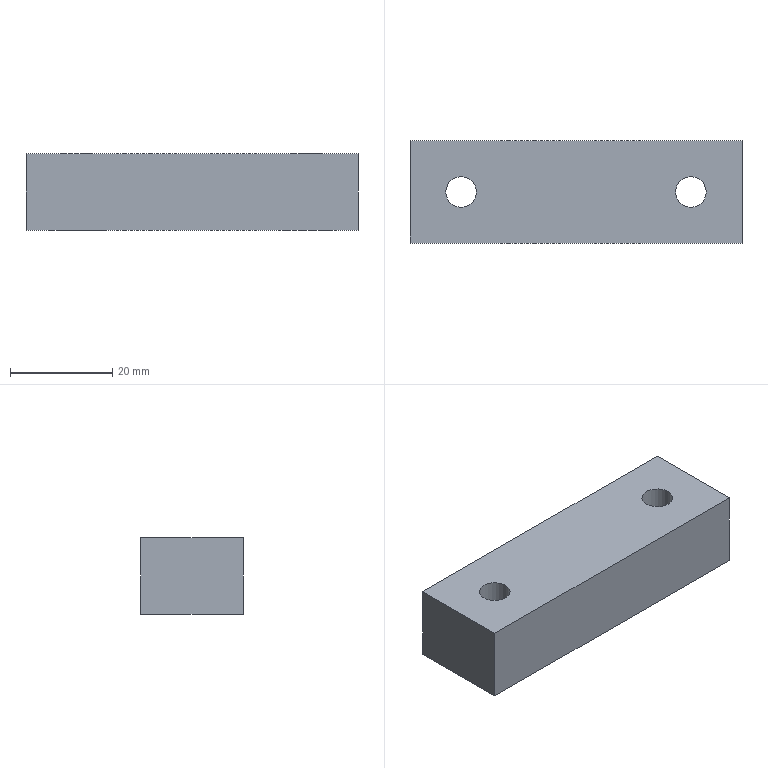Part | STEP file | gslz 2016.10.28-10_id2114_x_t | 1 solid | 12 faces | box 65 x 20 x 15 mm | volume 17584 mm3 | plane 8 | cylinder 4 | commonest cylinder face diameters 6 x2 11 x2
STEP:
#1=CARTESIAN_POINT('',(0.,0.,0.));
#2=DIRECTION('',(0.,0.,1.));
#3=DIRECTION('',(1.,0.,0.));
#4=AXIS2_PLACEMENT_3D('',#1,#2,#3);
#5=CARTESIAN_POINT('',(-46.5,-250.,28.));
#6=VERTEX_POINT('',#5);
#7=CARTESIAN_POINT('',(-41.,-250.,28.));
#8=DIRECTION('',(0.,0.,-1.));
#9=DIRECTION('',(-1.,0.,0.));
#10=AXIS2_PLACEMENT_3D('',#7,#8,#9);
#11=CIRCLE('',#10,5.5);
#12=CARTESIAN_POINT('',(-41.,-250.,30.));
#13=DIRECTION('',(0.,0.,-1.));
#14=DIRECTION('',(-1.,0.,0.));
#15=AXIS2_PLACEMENT_3D('',#12,#13,#14);
#16=CYLINDRICAL_SURFACE('',#15,5.5);
#17=CARTESIAN_POINT('',(0.,2.));
#18=DIRECTION('',(1.,0.));
#19=VECTOR('',#18,1.);
#20=LINE('',#17,#19);
#21=(GEOMETRIC_REPRESENTATION_CONTEXT(2)PARAMETRIC_REPRESENTATION_CONTEXT()REPRESENTATION_CONTEXT('',''));
#22=DEFINITIONAL_REPRESENTATION('',(#20),#21);
#23=PCURVE('',#16,#22);
#24=CARTESIAN_POINT('',(-3.5,-250.,28.));
#25=DIRECTION('',(0.,0.,-1.));
#26=DIRECTION('',(1.,0.,0.));
#27=AXIS2_PLACEMENT_3D('',#24,#25,#26);
#28=PLANE('',#27);
#29=CARTESIAN_POINT('',(-37.5,0.));
#30=DIRECTION('',(-1.,0.));
#31=AXIS2_PLACEMENT_2D('',#29,#30);
#32=CIRCLE('',#31,5.5);
#33=(GEOMETRIC_REPRESENTATION_CONTEXT(2)PARAMETRIC_REPRESENTATION_CONTEXT()REPRESENTATION_CONTEXT('',''));
#34=DEFINITIONAL_REPRESENTATION('',(#32),#33);
#35=PCURVE('',#28,#34);
#36=SURFACE_CURVE('',#11,(#23,#35),.PCURVE_S1.);
#37=EDGE_CURVE('',#6,#6,#36,.T.);
#38=ORIENTED_EDGE('',*,*,#37,.T.);
#39=CARTESIAN_POINT('',(-46.5,-250.,20.));
#40=VERTEX_POINT('',#39);
#41=CARTESIAN_POINT('',(-46.5,-250.,28.));
#42=CARTESIAN_POINT('',(-46.5,-250.,20.));
#43=B_SPLINE_CURVE_WITH_KNOTS('',1,(#41,#42),.UNSPECIFIED.,.F.,.F.,(2,2),(2.,10.),.PIECEWISE_BEZIER_KNOTS.);
#44=CARTESIAN_POINT('',(6.283,0.));
#45=DIRECTION('',(0.,1.));
#46=VECTOR('',#45,1.);
#47=LINE('',#44,#46);
#48=(GEOMETRIC_REPRESENTATION_CONTEXT(2)PARAMETRIC_REPRESENTATION_CONTEXT()REPRESENTATION_CONTEXT('',''));
#49=DEFINITIONAL_REPRESENTATION('',(#47),#48);
#50=PCURVE('',#16,#49);
#51=CARTESIAN_POINT('',(0.,0.));
#52=DIRECTION('',(0.,1.));
#53=VECTOR('',#52,1.);
#54=LINE('',#51,#53);
#55=(GEOMETRIC_REPRESENTATION_CONTEXT(2)PARAMETRIC_REPRESENTATION_CONTEXT()REPRESENTATION_CONTEXT('',''));
#56=DEFINITIONAL_REPRESENTATION('',(#54),#55);
#57=PCURVE('',#16,#56);
#58=SEAM_CURVE('',#43,(#50,#57),.PCURVE_S1.);
#59=EDGE_CURVE('',#6,#40,#58,.T.);
#60=ORIENTED_EDGE('',*,*,#59,.T.);
#61=CARTESIAN_POINT('',(-35.5,-250.,20.));
#62=VERTEX_POINT('',#61);
#63=CARTESIAN_POINT('',(-41.,-250.,20.));
#64=DIRECTION('',(0.,0.,-1.));
#65=DIRECTION('',(1.,0.,0.));
#66=AXIS2_PLACEMENT_3D('',#63,#64,#65);
#67=CIRCLE('',#66,5.5);
#68=CARTESIAN_POINT('',(3.142,10.));
#69=DIRECTION('',(1.,0.));
#70=VECTOR('',#69,1.);
#71=LINE('',#68,#70);
#72=(GEOMETRIC_REPRESENTATION_CONTEXT(2)PARAMETRIC_REPRESENTATION_CONTEXT()REPRESENTATION_CONTEXT('',''));
#73=DEFINITIONAL_REPRESENTATION('',(#71),#72);
#74=PCURVE('',#16,#73);
#75=CARTESIAN_POINT('',(-193.5,-250.,20.));
#76=DIRECTION('',(0.,0.,1.));
#77=DIRECTION('',(1.,0.,0.));
#78=AXIS2_PLACEMENT_3D('',#75,#76,#77);
#79=PLANE('',#78);
#80=CARTESIAN_POINT('',(158.,0.));
#81=CARTESIAN_POINT('',(158.,-9.526));
#82=CARTESIAN_POINT('',(149.75,-4.763));
#83=CARTESIAN_POINT('',(141.5,0.));
#84=CARTESIAN_POINT('',(149.75,4.763));
#85=CARTESIAN_POINT('',(158.,9.526));
#86=CARTESIAN_POINT('',(158.,0.));
#87=(BOUNDED_CURVE()B_SPLINE_CURVE(2,(#80,#81,#82,#83,#84,#85,#86),.UNSPECIFIED.,.T.,.F.)B_SPLINE_CURVE_WITH_KNOTS((1,2,2,2,2,1),(-2.094,0.,2.094,4.189,6.283,8.378),.UNSPECIFIED.)CURVE()GEOMETRIC_REPRESENTATION_ITEM()RATIONAL_B_SPLINE_CURVE((1.,0.5,1.,0.5,1.,0.5,1.))REPRESENTATION_ITEM(''));
#88=(GEOMETRIC_REPRESENTATION_CONTEXT(2)PARAMETRIC_REPRESENTATION_CONTEXT()REPRESENTATION_CONTEXT('',''));
#89=DEFINITIONAL_REPRESENTATION('',(#87),#88);
#90=PCURVE('',#79,#89);
#91=SURFACE_CURVE('',#67,(#74,#90),.PCURVE_S1.);
#92=EDGE_CURVE('',#62,#40,#91,.T.);
#93=ORIENTED_EDGE('',*,*,#92,.F.);
#94=CARTESIAN_POINT('',(-41.,-250.,20.));
#95=DIRECTION('',(0.,0.,-1.));
#96=DIRECTION('',(1.,0.,0.));
#97=AXIS2_PLACEMENT_3D('',#94,#95,#96);
#98=CIRCLE('',#97,5.5);
#99=CARTESIAN_POINT('',(-3.142,10.));
#100=DIRECTION('',(1.,0.));
#101=VECTOR('',#100,1.);
#102=LINE('',#99,#101);
#103=(GEOMETRIC_REPRESENTATION_CONTEXT(2)PARAMETRIC_REPRESENTATION_CONTEXT()REPRESENTATION_CONTEXT('',''));
#104=DEFINITIONAL_REPRESENTATION('',(#102),#103);
#105=PCURVE('',#16,#104);
#106=CARTESIAN_POINT('',(158.,0.));
#107=CARTESIAN_POINT('',(158.,-9.526));
#108=CARTESIAN_POINT('',(149.75,-4.763));
#109=CARTESIAN_POINT('',(141.5,0.));
#110=CARTESIAN_POINT('',(149.75,4.763));
#111=CARTESIAN_POINT('',(158.,9.526));
#112=CARTESIAN_POINT('',(158.,0.));
#113=(BOUNDED_CURVE()B_SPLINE_CURVE(2,(#106,#107,#108,#109,#110,#111,#112),.UNSPECIFIED.,.T.,.F.)B_SPLINE_CURVE_WITH_KNOTS((1,2,2,2,2,1),(-2.094,0.,2.094,4.189,6.283,8.378),.UNSPECIFIED.)CURVE()GEOMETRIC_REPRESENTATION_ITEM()RATIONAL_B_SPLINE_CURVE((1.,0.5,1.,0.5,1.,0.5,1.))REPRESENTATION_ITEM(''));
#114=(GEOMETRIC_REPRESENTATION_CONTEXT(2)PARAMETRIC_REPRESENTATION_CONTEXT()REPRESENTATION_CONTEXT('',''));
#115=DEFINITIONAL_REPRESENTATION('',(#113),#114);
#116=PCURVE('',#79,#115);
#117=SURFACE_CURVE('',#98,(#105,#116),.PCURVE_S1.);
#118=EDGE_CURVE('',#40,#62,#117,.T.);
#119=ORIENTED_EDGE('',*,*,#118,.F.);
#120=ORIENTED_EDGE('',*,*,#59,.F.);
#121=EDGE_LOOP('',(#38,#60,#93,#119,#120));
#122=FACE_BOUND('',#121,.F.);
#123=ADVANCED_FACE('',(#122),#16,.F.);
#124=CARTESIAN_POINT('',(-51.,-260.,35.));
#125=VERTEX_POINT('',#124);
#126=CARTESIAN_POINT('',(-51.,-260.,20.));
#127=VERTEX_POINT('',#126);
#128=CARTESIAN_POINT('',(-51.,-260.,30.));
#129=DIRECTION('',(0.,0.,-1.));
#130=VECTOR('',#129,1.);
#131=LINE('',#128,#130);
#132=CARTESIAN_POINT('',(-73.5,-260.,30.));
#133=DIRECTION('',(0.,1.,0.));
#134=DIRECTION('',(0.,0.,-1.));
#135=AXIS2_PLACEMENT_3D('',#132,#133,#134);
#136=PLANE('',#135);
#137=CARTESIAN_POINT('',(0.,-22.5));
#138=DIRECTION('',(1.,0.));
#139=VECTOR('',#138,1.);
#140=LINE('',#137,#139);
#141=(GEOMETRIC_REPRESENTATION_CONTEXT(2)PARAMETRIC_REPRESENTATION_CONTEXT()REPRESENTATION_CONTEXT('',''));
#142=DEFINITIONAL_REPRESENTATION('',(#140),#141);
#143=PCURVE('',#136,#142);
#144=CARTESIAN_POINT('',(-51.,-262.5,30.));
#145=DIRECTION('',(1.,0.,0.));
#146=DIRECTION('',(0.,0.,-1.));
#147=AXIS2_PLACEMENT_3D('',#144,#145,#146);
#148=PLANE('',#147);
#149=CARTESIAN_POINT('',(0.,2.5));
#150=DIRECTION('',(1.,0.));
#151=VECTOR('',#150,1.);
#152=LINE('',#149,#151);
#153=(GEOMETRIC_REPRESENTATION_CONTEXT(2)PARAMETRIC_REPRESENTATION_CONTEXT()REPRESENTATION_CONTEXT('',''));
#154=DEFINITIONAL_REPRESENTATION('',(#152),#153);
#155=PCURVE('',#148,#154);
#156=SURFACE_CURVE('',#131,(#143,#155),.PCURVE_S1.);
#157=EDGE_CURVE('',#125,#127,#156,.T.);
#158=ORIENTED_EDGE('',*,*,#157,.T.);
#159=CARTESIAN_POINT('',(14.,-260.,20.));
#160=VERTEX_POINT('',#159);
#161=CARTESIAN_POINT('',(-193.5,-260.,20.));
#162=DIRECTION('',(-1.,0.,0.));
#163=VECTOR('',#162,1.);
#164=LINE('',#161,#163);
#165=CARTESIAN_POINT('',(10.,120.));
#166=DIRECTION('',(0.,1.));
#167=VECTOR('',#166,1.);
#168=LINE('',#165,#167);
#169=(GEOMETRIC_REPRESENTATION_CONTEXT(2)PARAMETRIC_REPRESENTATION_CONTEXT()REPRESENTATION_CONTEXT('',''));
#170=DEFINITIONAL_REPRESENTATION('',(#168),#169);
#171=PCURVE('',#136,#170);
#172=CARTESIAN_POINT('',(0.,-10.));
#173=DIRECTION('',(-1.,0.));
#174=VECTOR('',#173,1.);
#175=LINE('',#172,#174);
#176=(GEOMETRIC_REPRESENTATION_CONTEXT(2)PARAMETRIC_REPRESENTATION_CONTEXT()REPRESENTATION_CONTEXT('',''));
#177=DEFINITIONAL_REPRESENTATION('',(#175),#176);
#178=PCURVE('',#79,#177);
#179=SURFACE_CURVE('',#164,(#171,#178),.PCURVE_S1.);
#180=EDGE_CURVE('',#160,#127,#179,.T.);
#181=ORIENTED_EDGE('',*,*,#180,.F.);
#182=CARTESIAN_POINT('',(14.,-260.,35.));
#183=VERTEX_POINT('',#182);
#184=CARTESIAN_POINT('',(14.,-260.,30.));
#185=DIRECTION('',(0.,0.,-1.));
#186=VECTOR('',#185,1.);
#187=LINE('',#184,#186);
#188=CARTESIAN_POINT('',(0.,-87.5));
#189=DIRECTION('',(1.,0.));
#190=VECTOR('',#189,1.);
#191=LINE('',#188,#190);
#192=(GEOMETRIC_REPRESENTATION_CONTEXT(2)PARAMETRIC_REPRESENTATION_CONTEXT()REPRESENTATION_CONTEXT('',''));
#193=DEFINITIONAL_REPRESENTATION('',(#191),#192);
#194=PCURVE('',#136,#193);
#195=CARTESIAN_POINT('',(14.,-237.5,30.));
#196=DIRECTION('',(-1.,0.,0.));
#197=DIRECTION('',(0.,0.,1.));
#198=AXIS2_PLACEMENT_3D('',#195,#196,#197);
#199=PLANE('',#198);
#200=CARTESIAN_POINT('',(0.,-22.5));
#201=DIRECTION('',(-1.,0.));
#202=VECTOR('',#201,1.);
#203=LINE('',#200,#202);
#204=(GEOMETRIC_REPRESENTATION_CONTEXT(2)PARAMETRIC_REPRESENTATION_CONTEXT()REPRESENTATION_CONTEXT('',''));
#205=DEFINITIONAL_REPRESENTATION('',(#203),#204);
#206=PCURVE('',#199,#205);
#207=SURFACE_CURVE('',#187,(#194,#206),.PCURVE_S1.);
#208=EDGE_CURVE('',#183,#160,#207,.T.);
#209=ORIENTED_EDGE('',*,*,#208,.F.);
#210=CARTESIAN_POINT('',(-193.5,-260.,35.));
#211=DIRECTION('',(-1.,0.,0.));
#212=VECTOR('',#211,1.);
#213=LINE('',#210,#212);
#214=CARTESIAN_POINT('',(-5.,120.));
#215=DIRECTION('',(0.,1.));
#216=VECTOR('',#215,1.);
#217=LINE('',#214,#216);
#218=(GEOMETRIC_REPRESENTATION_CONTEXT(2)PARAMETRIC_REPRESENTATION_CONTEXT()REPRESENTATION_CONTEXT('',''));
#219=DEFINITIONAL_REPRESENTATION('',(#217),#218);
#220=PCURVE('',#136,#219);
#221=CARTESIAN_POINT('',(-193.5,-250.,35.));
#222=DIRECTION('',(0.,0.,1.));
#223=DIRECTION('',(1.,0.,0.));
#224=AXIS2_PLACEMENT_3D('',#221,#222,#223);
#225=PLANE('',#224);
#226=CARTESIAN_POINT('',(0.,-10.));
#227=DIRECTION('',(-1.,0.));
#228=VECTOR('',#227,1.);
#229=LINE('',#226,#228);
#230=(GEOMETRIC_REPRESENTATION_CONTEXT(2)PARAMETRIC_REPRESENTATION_CONTEXT()REPRESENTATION_CONTEXT('',''));
#231=DEFINITIONAL_REPRESENTATION('',(#229),#230);
#232=PCURVE('',#225,#231);
#233=SURFACE_CURVE('',#213,(#220,#232),.PCURVE_S1.);
#234=EDGE_CURVE('',#183,#125,#233,.T.);
#235=ORIENTED_EDGE('',*,*,#234,.T.);
#236=EDGE_LOOP('',(#158,#181,#209,#235));
#237=FACE_BOUND('',#236,.T.);
#238=ADVANCED_FACE('',(#237),#136,.F.);
#239=ORIENTED_EDGE('',*,*,#208,.T.);
#240=CARTESIAN_POINT('',(14.,-240.,20.));
#241=VERTEX_POINT('',#240);
#242=CARTESIAN_POINT('',(14.,-237.5,20.));
#243=DIRECTION('',(0.,-1.,0.));
#244=VECTOR('',#243,1.);
#245=LINE('',#242,#244);
#246=CARTESIAN_POINT('',(-10.,0.));
#247=DIRECTION('',(0.,-1.));
#248=VECTOR('',#247,1.);
#249=LINE('',#246,#248);
#250=(GEOMETRIC_REPRESENTATION_CONTEXT(2)PARAMETRIC_REPRESENTATION_CONTEXT()REPRESENTATION_CONTEXT('',''));
#251=DEFINITIONAL_REPRESENTATION('',(#249),#250);
#252=PCURVE('',#199,#251);
#253=CARTESIAN_POINT('',(207.5,12.5));
#254=DIRECTION('',(0.,-1.));
#255=VECTOR('',#254,1.);
#256=LINE('',#253,#255);
#257=(GEOMETRIC_REPRESENTATION_CONTEXT(2)PARAMETRIC_REPRESENTATION_CONTEXT()REPRESENTATION_CONTEXT('',''));
#258=DEFINITIONAL_REPRESENTATION('',(#256),#257);
#259=PCURVE('',#79,#258);
#260=SURFACE_CURVE('',#245,(#252,#259),.PCURVE_S1.);
#261=EDGE_CURVE('',#241,#160,#260,.T.);
#262=ORIENTED_EDGE('',*,*,#261,.F.);
#263=CARTESIAN_POINT('',(14.,-240.,35.));
#264=VERTEX_POINT('',#263);
#265=CARTESIAN_POINT('',(14.,-240.,30.));
#266=DIRECTION('',(0.,0.,-1.));
#267=VECTOR('',#266,1.);
#268=LINE('',#265,#267);
#269=CARTESIAN_POINT('',(0.,-2.5));
#270=DIRECTION('',(-1.,0.));
#271=VECTOR('',#270,1.);
#272=LINE('',#269,#271);
#273=(GEOMETRIC_REPRESENTATION_CONTEXT(2)PARAMETRIC_REPRESENTATION_CONTEXT()REPRESENTATION_CONTEXT('',''));
#274=DEFINITIONAL_REPRESENTATION('',(#272),#273);
#275=PCURVE('',#199,#274);
#276=CARTESIAN_POINT('',(-203.5,-240.,30.));
#277=DIRECTION('',(0.,-1.,0.));
#278=DIRECTION('',(0.,0.,1.));
#279=AXIS2_PLACEMENT_3D('',#276,#277,#278);
#280=PLANE('',#279);
#281=CARTESIAN_POINT('',(0.,-217.5));
#282=DIRECTION('',(-1.,0.));
#283=VECTOR('',#282,1.);
#284=LINE('',#281,#283);
#285=(GEOMETRIC_REPRESENTATION_CONTEXT(2)PARAMETRIC_REPRESENTATION_CONTEXT()REPRESENTATION_CONTEXT('',''));
#286=DEFINITIONAL_REPRESENTATION('',(#284),#285);
#287=PCURVE('',#280,#286);
#288=SURFACE_CURVE('',#268,(#275,#287),.PCURVE_S1.);
#289=EDGE_CURVE('',#264,#241,#288,.T.);
#290=ORIENTED_EDGE('',*,*,#289,.F.);
#291=CARTESIAN_POINT('',(14.,-237.5,35.));
#292=DIRECTION('',(0.,-1.,0.));
#293=VECTOR('',#292,1.);
#294=LINE('',#291,#293);
#295=CARTESIAN_POINT('',(5.,0.));
#296=DIRECTION('',(0.,-1.));
#297=VECTOR('',#296,1.);
#298=LINE('',#295,#297);
#299=(GEOMETRIC_REPRESENTATION_CONTEXT(2)PARAMETRIC_REPRESENTATION_CONTEXT()REPRESENTATION_CONTEXT('',''));
#300=DEFINITIONAL_REPRESENTATION('',(#298),#299);
#301=PCURVE('',#199,#300);
#302=CARTESIAN_POINT('',(207.5,12.5));
#303=DIRECTION('',(0.,-1.));
#304=VECTOR('',#303,1.);
#305=LINE('',#302,#304);
#306=(GEOMETRIC_REPRESENTATION_CONTEXT(2)PARAMETRIC_REPRESENTATION_CONTEXT()REPRESENTATION_CONTEXT('',''));
#307=DEFINITIONAL_REPRESENTATION('',(#305),#306);
#308=PCURVE('',#225,#307);
#309=SURFACE_CURVE('',#294,(#301,#308),.PCURVE_S1.);
#310=EDGE_CURVE('',#264,#183,#309,.T.);
#311=ORIENTED_EDGE('',*,*,#310,.T.);
#312=EDGE_LOOP('',(#239,#262,#290,#311));
#313=FACE_BOUND('',#312,.T.);
#314=ADVANCED_FACE('',(#313),#199,.F.);
#315=ORIENTED_EDGE('',*,*,#289,.T.);
#316=CARTESIAN_POINT('',(-51.,-240.,20.));
#317=VERTEX_POINT('',#316);
#318=CARTESIAN_POINT('',(-193.5,-240.,20.));
#319=DIRECTION('',(1.,0.,0.));
#320=VECTOR('',#319,1.);
#321=LINE('',#318,#320);
#322=CARTESIAN_POINT('',(-10.,-10.));
#323=DIRECTION('',(0.,-1.));
#324=VECTOR('',#323,1.);
#325=LINE('',#322,#324);
#326=(GEOMETRIC_REPRESENTATION_CONTEXT(2)PARAMETRIC_REPRESENTATION_CONTEXT()REPRESENTATION_CONTEXT('',''));
#327=DEFINITIONAL_REPRESENTATION('',(#325),#326);
#328=PCURVE('',#280,#327);
#329=CARTESIAN_POINT('',(0.,10.));
#330=DIRECTION('',(1.,0.));
#331=VECTOR('',#330,1.);
#332=LINE('',#329,#331);
#333=(GEOMETRIC_REPRESENTATION_CONTEXT(2)PARAMETRIC_REPRESENTATION_CONTEXT()REPRESENTATION_CONTEXT('',''));
#334=DEFINITIONAL_REPRESENTATION('',(#332),#333);
#335=PCURVE('',#79,#334);
#336=SURFACE_CURVE('',#321,(#328,#335),.PCURVE_S1.);
#337=EDGE_CURVE('',#317,#241,#336,.T.);
#338=ORIENTED_EDGE('',*,*,#337,.F.);
#339=CARTESIAN_POINT('',(-51.,-240.,35.));
#340=VERTEX_POINT('',#339);
#341=CARTESIAN_POINT('',(-51.,-240.,30.));
#342=DIRECTION('',(0.,0.,-1.));
#343=VECTOR('',#342,1.);
#344=LINE('',#341,#343);
#345=CARTESIAN_POINT('',(0.,-152.5));
#346=DIRECTION('',(-1.,0.));
#347=VECTOR('',#346,1.);
#348=LINE('',#345,#347);
#349=(GEOMETRIC_REPRESENTATION_CONTEXT(2)PARAMETRIC_REPRESENTATION_CONTEXT()REPRESENTATION_CONTEXT('',''));
#350=DEFINITIONAL_REPRESENTATION('',(#348),#349);
#351=PCURVE('',#280,#350);
#352=CARTESIAN_POINT('',(0.,22.5));
#353=DIRECTION('',(1.,0.));
#354=VECTOR('',#353,1.);
#355=LINE('',#352,#354);
#356=(GEOMETRIC_REPRESENTATION_CONTEXT(2)PARAMETRIC_REPRESENTATION_CONTEXT()REPRESENTATION_CONTEXT('',''));
#357=DEFINITIONAL_REPRESENTATION('',(#355),#356);
#358=PCURVE('',#148,#357);
#359=SURFACE_CURVE('',#344,(#351,#358),.PCURVE_S1.);
#360=EDGE_CURVE('',#340,#317,#359,.T.);
#361=ORIENTED_EDGE('',*,*,#360,.F.);
#362=CARTESIAN_POINT('',(-193.5,-240.,35.));
#363=DIRECTION('',(1.,0.,0.));
#364=VECTOR('',#363,1.);
#365=LINE('',#362,#364);
#366=CARTESIAN_POINT('',(5.,-10.));
#367=DIRECTION('',(0.,-1.));
#368=VECTOR('',#367,1.);
#369=LINE('',#366,#368);
#370=(GEOMETRIC_REPRESENTATION_CONTEXT(2)PARAMETRIC_REPRESENTATION_CONTEXT()REPRESENTATION_CONTEXT('',''));
#371=DEFINITIONAL_REPRESENTATION('',(#369),#370);
#372=PCURVE('',#280,#371);
#373=CARTESIAN_POINT('',(0.,10.));
#374=DIRECTION('',(1.,0.));
#375=VECTOR('',#374,1.);
#376=LINE('',#373,#375);
#377=(GEOMETRIC_REPRESENTATION_CONTEXT(2)PARAMETRIC_REPRESENTATION_CONTEXT()REPRESENTATION_CONTEXT('',''));
#378=DEFINITIONAL_REPRESENTATION('',(#376),#377);
#379=PCURVE('',#225,#378);
#380=SURFACE_CURVE('',#365,(#372,#379),.PCURVE_S1.);
#381=EDGE_CURVE('',#340,#264,#380,.T.);
#382=ORIENTED_EDGE('',*,*,#381,.T.);
#383=EDGE_LOOP('',(#315,#338,#361,#382));
#384=FACE_BOUND('',#383,.T.);
#385=ADVANCED_FACE('',(#384),#280,.F.);
#386=ORIENTED_EDGE('',*,*,#360,.T.);
#387=CARTESIAN_POINT('',(-51.,-262.5,20.));
#388=DIRECTION('',(0.,1.,0.));
#389=VECTOR('',#388,1.);
#390=LINE('',#387,#389);
#391=CARTESIAN_POINT('',(10.,0.));
#392=DIRECTION('',(0.,1.));
#393=VECTOR('',#392,1.);
#394=LINE('',#391,#393);
#395=(GEOMETRIC_REPRESENTATION_CONTEXT(2)PARAMETRIC_REPRESENTATION_CONTEXT()REPRESENTATION_CONTEXT('',''));
#396=DEFINITIONAL_REPRESENTATION('',(#394),#395);
#397=PCURVE('',#148,#396);
#398=CARTESIAN_POINT('',(142.5,-12.5));
#399=DIRECTION('',(0.,1.));
#400=VECTOR('',#399,1.);
#401=LINE('',#398,#400);
#402=(GEOMETRIC_REPRESENTATION_CONTEXT(2)PARAMETRIC_REPRESENTATION_CONTEXT()REPRESENTATION_CONTEXT('',''));
#403=DEFINITIONAL_REPRESENTATION('',(#401),#402);
#404=PCURVE('',#79,#403);
#405=SURFACE_CURVE('',#390,(#397,#404),.PCURVE_S1.);
#406=EDGE_CURVE('',#127,#317,#405,.T.);
#407=ORIENTED_EDGE('',*,*,#406,.F.);
#408=ORIENTED_EDGE('',*,*,#157,.F.);
#409=CARTESIAN_POINT('',(-51.,-262.5,35.));
#410=DIRECTION('',(0.,1.,0.));
#411=VECTOR('',#410,1.);
#412=LINE('',#409,#411);
#413=CARTESIAN_POINT('',(-5.,0.));
#414=DIRECTION('',(0.,1.));
#415=VECTOR('',#414,1.);
#416=LINE('',#413,#415);
#417=(GEOMETRIC_REPRESENTATION_CONTEXT(2)PARAMETRIC_REPRESENTATION_CONTEXT()REPRESENTATION_CONTEXT('',''));
#418=DEFINITIONAL_REPRESENTATION('',(#416),#417);
#419=PCURVE('',#148,#418);
#420=CARTESIAN_POINT('',(142.5,-12.5));
#421=DIRECTION('',(0.,1.));
#422=VECTOR('',#421,1.);
#423=LINE('',#420,#422);
#424=(GEOMETRIC_REPRESENTATION_CONTEXT(2)PARAMETRIC_REPRESENTATION_CONTEXT()REPRESENTATION_CONTEXT('',''));
#425=DEFINITIONAL_REPRESENTATION('',(#423),#424);
#426=PCURVE('',#225,#425);
#427=SURFACE_CURVE('',#412,(#419,#426),.PCURVE_S1.);
#428=EDGE_CURVE('',#125,#340,#427,.T.);
#429=ORIENTED_EDGE('',*,*,#428,.T.);
#430=EDGE_LOOP('',(#386,#407,#408,#429));
#431=FACE_BOUND('',#430,.T.);
#432=ADVANCED_FACE('',(#431),#148,.F.);
#433=ORIENTED_EDGE('',*,*,#406,.T.);
#434=ORIENTED_EDGE('',*,*,#337,.T.);
#435=ORIENTED_EDGE('',*,*,#261,.T.);
#436=ORIENTED_EDGE('',*,*,#180,.T.);
#437=EDGE_LOOP('',(#433,#434,#435,#436));
#438=FACE_BOUND('',#437,.T.);
#439=ORIENTED_EDGE('',*,*,#92,.F.);
#440=ORIENTED_EDGE('',*,*,#118,.F.);
#441=EDGE_LOOP('',(#439,#440));
#442=FACE_BOUND('',#441,.T.);
#443=CARTESIAN_POINT('',(9.5,-250.,20.));
#444=VERTEX_POINT('',#443);
#445=CARTESIAN_POINT('',(-1.5,-250.,20.));
#446=VERTEX_POINT('',#445);
#447=CARTESIAN_POINT('',(4.,-250.,20.));
#448=DIRECTION('',(0.,0.,-1.));
#449=DIRECTION('',(1.,0.,0.));
#450=AXIS2_PLACEMENT_3D('',#447,#448,#449);
#451=CIRCLE('',#450,5.5);
#452=CARTESIAN_POINT('',(203.,0.));
#453=CARTESIAN_POINT('',(203.,-9.526));
#454=CARTESIAN_POINT('',(194.75,-4.763));
#455=CARTESIAN_POINT('',(186.5,0.));
#456=CARTESIAN_POINT('',(194.75,4.763));
#457=CARTESIAN_POINT('',(203.,9.526));
#458=CARTESIAN_POINT('',(203.,0.));
#459=(BOUNDED_CURVE()B_SPLINE_CURVE(2,(#452,#453,#454,#455,#456,#457,#458),.UNSPECIFIED.,.T.,.F.)B_SPLINE_CURVE_WITH_KNOTS((1,2,2,2,2,1),(-2.094,0.,2.094,4.189,6.283,8.378),.UNSPECIFIED.)CURVE()GEOMETRIC_REPRESENTATION_ITEM()RATIONAL_B_SPLINE_CURVE((1.,0.5,1.,0.5,1.,0.5,1.))REPRESENTATION_ITEM(''));
#460=(GEOMETRIC_REPRESENTATION_CONTEXT(2)PARAMETRIC_REPRESENTATION_CONTEXT()REPRESENTATION_CONTEXT('',''));
#461=DEFINITIONAL_REPRESENTATION('',(#459),#460);
#462=PCURVE('',#79,#461);
#463=CARTESIAN_POINT('',(4.,-250.,30.));
#464=DIRECTION('',(0.,0.,-1.));
#465=DIRECTION('',(-1.,0.,0.));
#466=AXIS2_PLACEMENT_3D('',#463,#464,#465);
#467=CYLINDRICAL_SURFACE('',#466,5.5);
#468=CARTESIAN_POINT('',(3.142,10.));
#469=DIRECTION('',(1.,0.));
#470=VECTOR('',#469,1.);
#471=LINE('',#468,#470);
#472=(GEOMETRIC_REPRESENTATION_CONTEXT(2)PARAMETRIC_REPRESENTATION_CONTEXT()REPRESENTATION_CONTEXT('',''));
#473=DEFINITIONAL_REPRESENTATION('',(#471),#472);
#474=PCURVE('',#467,#473);
#475=SURFACE_CURVE('',#451,(#462,#474),.PCURVE_S1.);
#476=EDGE_CURVE('',#444,#446,#475,.T.);
#477=ORIENTED_EDGE('',*,*,#476,.F.);
#478=CARTESIAN_POINT('',(4.,-250.,20.));
#479=DIRECTION('',(0.,0.,-1.));
#480=DIRECTION('',(1.,0.,0.));
#481=AXIS2_PLACEMENT_3D('',#478,#479,#480);
#482=CIRCLE('',#481,5.5);
#483=CARTESIAN_POINT('',(203.,0.));
#484=CARTESIAN_POINT('',(203.,-9.526));
#485=CARTESIAN_POINT('',(194.75,-4.763));
#486=CARTESIAN_POINT('',(186.5,0.));
#487=CARTESIAN_POINT('',(194.75,4.763));
#488=CARTESIAN_POINT('',(203.,9.526));
#489=CARTESIAN_POINT('',(203.,0.));
#490=(BOUNDED_CURVE()B_SPLINE_CURVE(2,(#483,#484,#485,#486,#487,#488,#489),.UNSPECIFIED.,.T.,.F.)B_SPLINE_CURVE_WITH_KNOTS((1,2,2,2,2,1),(-2.094,0.,2.094,4.189,6.283,8.378),.UNSPECIFIED.)CURVE()GEOMETRIC_REPRESENTATION_ITEM()RATIONAL_B_SPLINE_CURVE((1.,0.5,1.,0.5,1.,0.5,1.))REPRESENTATION_ITEM(''));
#491=(GEOMETRIC_REPRESENTATION_CONTEXT(2)PARAMETRIC_REPRESENTATION_CONTEXT()REPRESENTATION_CONTEXT('',''));
#492=DEFINITIONAL_REPRESENTATION('',(#490),#491);
#493=PCURVE('',#79,#492);
#494=CARTESIAN_POINT('',(-3.142,10.));
#495=DIRECTION('',(1.,0.));
#496=VECTOR('',#495,1.);
#497=LINE('',#494,#496);
#498=(GEOMETRIC_REPRESENTATION_CONTEXT(2)PARAMETRIC_REPRESENTATION_CONTEXT()REPRESENTATION_CONTEXT('',''));
#499=DEFINITIONAL_REPRESENTATION('',(#497),#498);
#500=PCURVE('',#467,#499);
#501=SURFACE_CURVE('',#482,(#493,#500),.PCURVE_S1.);
#502=EDGE_CURVE('',#446,#444,#501,.T.);
#503=ORIENTED_EDGE('',*,*,#502,.F.);
#504=EDGE_LOOP('',(#477,#503));
#505=FACE_BOUND('',#504,.T.);
#506=ADVANCED_FACE('',(#438,#442,#505),#79,.F.);
#507=CARTESIAN_POINT('',(-1.5,-250.,28.));
#508=VERTEX_POINT('',#507);
#509=CARTESIAN_POINT('',(4.,-250.,28.));
#510=DIRECTION('',(0.,0.,-1.));
#511=DIRECTION('',(-1.,0.,0.));
#512=AXIS2_PLACEMENT_3D('',#509,#510,#511);
#513=CIRCLE('',#512,5.5);
#514=CARTESIAN_POINT('',(0.,2.));
#515=DIRECTION('',(1.,0.));
#516=VECTOR('',#515,1.);
#517=LINE('',#514,#516);
#518=(GEOMETRIC_REPRESENTATION_CONTEXT(2)PARAMETRIC_REPRESENTATION_CONTEXT()REPRESENTATION_CONTEXT('',''));
#519=DEFINITIONAL_REPRESENTATION('',(#517),#518);
#520=PCURVE('',#467,#519);
#521=CARTESIAN_POINT('',(-33.5,-250.,28.));
#522=DIRECTION('',(0.,0.,-1.));
#523=DIRECTION('',(1.,0.,0.));
#524=AXIS2_PLACEMENT_3D('',#521,#522,#523);
#525=PLANE('',#524);
#526=CARTESIAN_POINT('',(37.5,0.));
#527=DIRECTION('',(-1.,0.));
#528=AXIS2_PLACEMENT_2D('',#526,#527);
#529=CIRCLE('',#528,5.5);
#530=(GEOMETRIC_REPRESENTATION_CONTEXT(2)PARAMETRIC_REPRESENTATION_CONTEXT()REPRESENTATION_CONTEXT('',''));
#531=DEFINITIONAL_REPRESENTATION('',(#529),#530);
#532=PCURVE('',#525,#531);
#533=SURFACE_CURVE('',#513,(#520,#532),.PCURVE_S1.);
#534=EDGE_CURVE('',#508,#508,#533,.T.);
#535=ORIENTED_EDGE('',*,*,#534,.T.);
#536=CARTESIAN_POINT('',(-1.5,-250.,28.));
#537=CARTESIAN_POINT('',(-1.5,-250.,20.));
#538=B_SPLINE_CURVE_WITH_KNOTS('',1,(#536,#537),.UNSPECIFIED.,.F.,.F.,(2,2),(2.,10.),.PIECEWISE_BEZIER_KNOTS.);
#539=CARTESIAN_POINT('',(6.283,0.));
#540=DIRECTION('',(0.,1.));
#541=VECTOR('',#540,1.);
#542=LINE('',#539,#541);
#543=(GEOMETRIC_REPRESENTATION_CONTEXT(2)PARAMETRIC_REPRESENTATION_CONTEXT()REPRESENTATION_CONTEXT('',''));
#544=DEFINITIONAL_REPRESENTATION('',(#542),#543);
#545=PCURVE('',#467,#544);
#546=CARTESIAN_POINT('',(0.,0.));
#547=DIRECTION('',(0.,1.));
#548=VECTOR('',#547,1.);
#549=LINE('',#546,#548);
#550=(GEOMETRIC_REPRESENTATION_CONTEXT(2)PARAMETRIC_REPRESENTATION_CONTEXT()REPRESENTATION_CONTEXT('',''));
#551=DEFINITIONAL_REPRESENTATION('',(#549),#550);
#552=PCURVE('',#467,#551);
#553=SEAM_CURVE('',#538,(#545,#552),.PCURVE_S1.);
#554=EDGE_CURVE('',#508,#446,#553,.T.);
#555=ORIENTED_EDGE('',*,*,#554,.T.);
#556=ORIENTED_EDGE('',*,*,#476,.F.);
#557=ORIENTED_EDGE('',*,*,#502,.F.);
#558=ORIENTED_EDGE('',*,*,#554,.F.);
#559=EDGE_LOOP('',(#535,#555,#556,#557,#558));
#560=FACE_BOUND('',#559,.F.);
#561=ADVANCED_FACE('',(#560),#467,.F.);
#562=CARTESIAN_POINT('',(1.,-250.,28.));
#563=VERTEX_POINT('',#562);
#564=CARTESIAN_POINT('',(4.,-250.,28.));
#565=DIRECTION('',(0.,0.,1.));
#566=DIRECTION('',(-1.,0.,0.));
#567=AXIS2_PLACEMENT_3D('',#564,#565,#566);
#568=CIRCLE('',#567,3.);
#569=CARTESIAN_POINT('',(34.5,0.));
#570=CARTESIAN_POINT('',(34.5,5.196));
#571=CARTESIAN_POINT('',(39.,2.598));
#572=CARTESIAN_POINT('',(43.5,0.));
#573=CARTESIAN_POINT('',(39.,-2.598));
#574=CARTESIAN_POINT('',(34.5,-5.196));
#575=CARTESIAN_POINT('',(34.5,0.));
#576=(BOUNDED_CURVE()B_SPLINE_CURVE(2,(#569,#570,#571,#572,#573,#574,#575),.UNSPECIFIED.,.T.,.F.)B_SPLINE_CURVE_WITH_KNOTS((1,2,2,2,2,1),(-2.094,0.,2.094,4.189,6.283,8.378),.UNSPECIFIED.)CURVE()GEOMETRIC_REPRESENTATION_ITEM()RATIONAL_B_SPLINE_CURVE((1.,0.5,1.,0.5,1.,0.5,1.))REPRESENTATION_ITEM(''));
#577=(GEOMETRIC_REPRESENTATION_CONTEXT(2)PARAMETRIC_REPRESENTATION_CONTEXT()REPRESENTATION_CONTEXT('',''));
#578=DEFINITIONAL_REPRESENTATION('',(#576),#577);
#579=PCURVE('',#525,#578);
#580=CARTESIAN_POINT('',(4.,-250.,30.));
#581=DIRECTION('',(0.,0.,-1.));
#582=DIRECTION('',(-1.,0.,0.));
#583=AXIS2_PLACEMENT_3D('',#580,#581,#582);
#584=CYLINDRICAL_SURFACE('',#583,3.);
#585=CARTESIAN_POINT('',(6.283,2.));
#586=DIRECTION('',(-1.,0.));
#587=VECTOR('',#586,1.);
#588=LINE('',#585,#587);
#589=(GEOMETRIC_REPRESENTATION_CONTEXT(2)PARAMETRIC_REPRESENTATION_CONTEXT()REPRESENTATION_CONTEXT('',''));
#590=DEFINITIONAL_REPRESENTATION('',(#588),#589);
#591=PCURVE('',#584,#590);
#592=SURFACE_CURVE('',#568,(#579,#591),.PCURVE_S1.);
#593=EDGE_CURVE('',#563,#563,#592,.T.);
#594=ORIENTED_EDGE('',*,*,#593,.T.);
#595=EDGE_LOOP('',(#594));
#596=FACE_BOUND('',#595,.T.);
#597=ORIENTED_EDGE('',*,*,#534,.T.);
#598=EDGE_LOOP('',(#597));
#599=FACE_BOUND('',#598,.T.);
#600=ADVANCED_FACE('',(#596,#599),#525,.T.);
#601=CARTESIAN_POINT('',(-44.,-250.,28.));
#602=VERTEX_POINT('',#601);
#603=CARTESIAN_POINT('',(-41.,-250.,28.));
#604=DIRECTION('',(0.,0.,1.));
#605=DIRECTION('',(-1.,0.,0.));
#606=AXIS2_PLACEMENT_3D('',#603,#604,#605);
#607=CIRCLE('',#606,3.);
#608=CARTESIAN_POINT('',(-40.5,0.));
#609=CARTESIAN_POINT('',(-40.5,5.196));
#610=CARTESIAN_POINT('',(-36.,2.598));
#611=CARTESIAN_POINT('',(-31.5,0.));
#612=CARTESIAN_POINT('',(-36.,-2.598));
#613=CARTESIAN_POINT('',(-40.5,-5.196));
#614=CARTESIAN_POINT('',(-40.5,0.));
#615=(BOUNDED_CURVE()B_SPLINE_CURVE(2,(#608,#609,#610,#611,#612,#613,#614),.UNSPECIFIED.,.T.,.F.)B_SPLINE_CURVE_WITH_KNOTS((1,2,2,2,2,1),(-2.094,0.,2.094,4.189,6.283,8.378),.UNSPECIFIED.)CURVE()GEOMETRIC_REPRESENTATION_ITEM()RATIONAL_B_SPLINE_CURVE((1.,0.5,1.,0.5,1.,0.5,1.))REPRESENTATION_ITEM(''));
#616=(GEOMETRIC_REPRESENTATION_CONTEXT(2)PARAMETRIC_REPRESENTATION_CONTEXT()REPRESENTATION_CONTEXT('',''));
#617=DEFINITIONAL_REPRESENTATION('',(#615),#616);
#618=PCURVE('',#28,#617);
#619=CARTESIAN_POINT('',(-41.,-250.,30.));
#620=DIRECTION('',(0.,0.,-1.));
#621=DIRECTION('',(-1.,0.,0.));
#622=AXIS2_PLACEMENT_3D('',#619,#620,#621);
#623=CYLINDRICAL_SURFACE('',#622,3.);
#624=CARTESIAN_POINT('',(6.283,2.));
#625=DIRECTION('',(-1.,0.));
#626=VECTOR('',#625,1.);
#627=LINE('',#624,#626);
#628=(GEOMETRIC_REPRESENTATION_CONTEXT(2)PARAMETRIC_REPRESENTATION_CONTEXT()REPRESENTATION_CONTEXT('',''));
#629=DEFINITIONAL_REPRESENTATION('',(#627),#628);
#630=PCURVE('',#623,#629);
#631=SURFACE_CURVE('',#607,(#618,#630),.PCURVE_S1.);
#632=EDGE_CURVE('',#602,#602,#631,.T.);
#633=ORIENTED_EDGE('',*,*,#632,.T.);
#634=EDGE_LOOP('',(#633));
#635=FACE_BOUND('',#634,.T.);
#636=ORIENTED_EDGE('',*,*,#37,.T.);
#637=EDGE_LOOP('',(#636));
#638=FACE_BOUND('',#637,.T.);
#639=ADVANCED_FACE('',(#635,#638),#28,.T.);
#640=CARTESIAN_POINT('',(-38.,-250.,35.));
#641=VERTEX_POINT('',#640);
#642=CARTESIAN_POINT('',(-44.,-250.,35.));
#643=VERTEX_POINT('',#642);
#644=CARTESIAN_POINT('',(-41.,-250.,35.));
#645=DIRECTION('',(0.,0.,-1.));
#646=DIRECTION('',(1.,0.,0.));
#647=AXIS2_PLACEMENT_3D('',#644,#645,#646);
#648=CIRCLE('',#647,3.);
#649=CARTESIAN_POINT('',(3.142,-5.));
#650=DIRECTION('',(1.,0.));
#651=VECTOR('',#650,1.);
#652=LINE('',#649,#651);
#653=(GEOMETRIC_REPRESENTATION_CONTEXT(2)PARAMETRIC_REPRESENTATION_CONTEXT()REPRESENTATION_CONTEXT('',''));
#654=DEFINITIONAL_REPRESENTATION('',(#652),#653);
#655=PCURVE('',#623,#654);
#656=CARTESIAN_POINT('',(155.5,0.));
#657=CARTESIAN_POINT('',(155.5,-5.196));
#658=CARTESIAN_POINT('',(151.,-2.598));
#659=CARTESIAN_POINT('',(146.5,0.));
#660=CARTESIAN_POINT('',(151.,2.598));
#661=CARTESIAN_POINT('',(155.5,5.196));
#662=CARTESIAN_POINT('',(155.5,0.));
#663=(BOUNDED_CURVE()B_SPLINE_CURVE(2,(#656,#657,#658,#659,#660,#661,#662),.UNSPECIFIED.,.T.,.F.)B_SPLINE_CURVE_WITH_KNOTS((1,2,2,2,2,1),(-2.094,0.,2.094,4.189,6.283,8.378),.UNSPECIFIED.)CURVE()GEOMETRIC_REPRESENTATION_ITEM()RATIONAL_B_SPLINE_CURVE((1.,0.5,1.,0.5,1.,0.5,1.))REPRESENTATION_ITEM(''));
#664=(GEOMETRIC_REPRESENTATION_CONTEXT(2)PARAMETRIC_REPRESENTATION_CONTEXT()REPRESENTATION_CONTEXT('',''));
#665=DEFINITIONAL_REPRESENTATION('',(#663),#664);
#666=PCURVE('',#225,#665);
#667=SURFACE_CURVE('',#648,(#655,#666),.PCURVE_S1.);
#668=EDGE_CURVE('',#641,#643,#667,.T.);
#669=ORIENTED_EDGE('',*,*,#668,.T.);
#670=CARTESIAN_POINT('',(-44.,-250.,35.));
#671=CARTESIAN_POINT('',(-44.,-250.,28.));
#672=B_SPLINE_CURVE_WITH_KNOTS('',1,(#670,#671),.UNSPECIFIED.,.F.,.F.,(2,2),(-5.,2.),.PIECEWISE_BEZIER_KNOTS.);
#673=CARTESIAN_POINT('',(6.283,0.));
#674=DIRECTION('',(0.,1.));
#675=VECTOR('',#674,1.);
#676=LINE('',#673,#675);
#677=(GEOMETRIC_REPRESENTATION_CONTEXT(2)PARAMETRIC_REPRESENTATION_CONTEXT()REPRESENTATION_CONTEXT('',''));
#678=DEFINITIONAL_REPRESENTATION('',(#676),#677);
#679=PCURVE('',#623,#678);
#680=CARTESIAN_POINT('',(0.,0.));
#681=DIRECTION('',(0.,1.));
#682=VECTOR('',#681,1.);
#683=LINE('',#680,#682);
#684=(GEOMETRIC_REPRESENTATION_CONTEXT(2)PARAMETRIC_REPRESENTATION_CONTEXT()REPRESENTATION_CONTEXT('',''));
#685=DEFINITIONAL_REPRESENTATION('',(#683),#684);
#686=PCURVE('',#623,#685);
#687=SEAM_CURVE('',#672,(#679,#686),.PCURVE_S1.);
#688=EDGE_CURVE('',#643,#602,#687,.T.);
#689=ORIENTED_EDGE('',*,*,#688,.T.);
#690=ORIENTED_EDGE('',*,*,#632,.T.);
#691=ORIENTED_EDGE('',*,*,#688,.F.);
#692=CARTESIAN_POINT('',(-41.,-250.,35.));
#693=DIRECTION('',(0.,0.,-1.));
#694=DIRECTION('',(1.,0.,0.));
#695=AXIS2_PLACEMENT_3D('',#692,#693,#694);
#696=CIRCLE('',#695,3.);
#697=CARTESIAN_POINT('',(-3.142,-5.));
#698=DIRECTION('',(1.,0.));
#699=VECTOR('',#698,1.);
#700=LINE('',#697,#699);
#701=(GEOMETRIC_REPRESENTATION_CONTEXT(2)PARAMETRIC_REPRESENTATION_CONTEXT()REPRESENTATION_CONTEXT('',''));
#702=DEFINITIONAL_REPRESENTATION('',(#700),#701);
#703=PCURVE('',#623,#702);
#704=CARTESIAN_POINT('',(155.5,0.));
#705=CARTESIAN_POINT('',(155.5,-5.196));
#706=CARTESIAN_POINT('',(151.,-2.598));
#707=CARTESIAN_POINT('',(146.5,0.));
#708=CARTESIAN_POINT('',(151.,2.598));
#709=CARTESIAN_POINT('',(155.5,5.196));
#710=CARTESIAN_POINT('',(155.5,0.));
#711=(BOUNDED_CURVE()B_SPLINE_CURVE(2,(#704,#705,#706,#707,#708,#709,#710),.UNSPECIFIED.,.T.,.F.)B_SPLINE_CURVE_WITH_KNOTS((1,2,2,2,2,1),(-2.094,0.,2.094,4.189,6.283,8.378),.UNSPECIFIED.)CURVE()GEOMETRIC_REPRESENTATION_ITEM()RATIONAL_B_SPLINE_CURVE((1.,0.5,1.,0.5,1.,0.5,1.))REPRESENTATION_ITEM(''));
#712=(GEOMETRIC_REPRESENTATION_CONTEXT(2)PARAMETRIC_REPRESENTATION_CONTEXT()REPRESENTATION_CONTEXT('',''));
#713=DEFINITIONAL_REPRESENTATION('',(#711),#712);
#714=PCURVE('',#225,#713);
#715=SURFACE_CURVE('',#696,(#703,#714),.PCURVE_S1.);
#716=EDGE_CURVE('',#643,#641,#715,.T.);
#717=ORIENTED_EDGE('',*,*,#716,.T.);
#718=EDGE_LOOP('',(#669,#689,#690,#691,#717));
#719=FACE_BOUND('',#718,.F.);
#720=ADVANCED_FACE('',(#719),#623,.F.);
#721=CARTESIAN_POINT('',(7.,-250.,35.));
#722=VERTEX_POINT('',#721);
#723=CARTESIAN_POINT('',(1.,-250.,35.));
#724=VERTEX_POINT('',#723);
#725=CARTESIAN_POINT('',(4.,-250.,35.));
#726=DIRECTION('',(0.,0.,-1.));
#727=DIRECTION('',(1.,0.,0.));
#728=AXIS2_PLACEMENT_3D('',#725,#726,#727);
#729=CIRCLE('',#728,3.);
#730=CARTESIAN_POINT('',(3.142,-5.));
#731=DIRECTION('',(1.,0.));
#732=VECTOR('',#731,1.);
#733=LINE('',#730,#732);
#734=(GEOMETRIC_REPRESENTATION_CONTEXT(2)PARAMETRIC_REPRESENTATION_CONTEXT()REPRESENTATION_CONTEXT('',''));
#735=DEFINITIONAL_REPRESENTATION('',(#733),#734);
#736=PCURVE('',#584,#735);
#737=CARTESIAN_POINT('',(200.5,0.));
#738=CARTESIAN_POINT('',(200.5,-5.196));
#739=CARTESIAN_POINT('',(196.,-2.598));
#740=CARTESIAN_POINT('',(191.5,0.));
#741=CARTESIAN_POINT('',(196.,2.598));
#742=CARTESIAN_POINT('',(200.5,5.196));
#743=CARTESIAN_POINT('',(200.5,0.));
#744=(BOUNDED_CURVE()B_SPLINE_CURVE(2,(#737,#738,#739,#740,#741,#742,#743),.UNSPECIFIED.,.T.,.F.)B_SPLINE_CURVE_WITH_KNOTS((1,2,2,2,2,1),(-2.094,0.,2.094,4.189,6.283,8.378),.UNSPECIFIED.)CURVE()GEOMETRIC_REPRESENTATION_ITEM()RATIONAL_B_SPLINE_CURVE((1.,0.5,1.,0.5,1.,0.5,1.))REPRESENTATION_ITEM(''));
#745=(GEOMETRIC_REPRESENTATION_CONTEXT(2)PARAMETRIC_REPRESENTATION_CONTEXT()REPRESENTATION_CONTEXT('',''));
#746=DEFINITIONAL_REPRESENTATION('',(#744),#745);
#747=PCURVE('',#225,#746);
#748=SURFACE_CURVE('',#729,(#736,#747),.PCURVE_S1.);
#749=EDGE_CURVE('',#722,#724,#748,.T.);
#750=ORIENTED_EDGE('',*,*,#749,.T.);
#751=CARTESIAN_POINT('',(1.,-250.,35.));
#752=CARTESIAN_POINT('',(1.,-250.,28.));
#753=B_SPLINE_CURVE_WITH_KNOTS('',1,(#751,#752),.UNSPECIFIED.,.F.,.F.,(2,2),(-5.,2.),.PIECEWISE_BEZIER_KNOTS.);
#754=CARTESIAN_POINT('',(6.283,0.));
#755=DIRECTION('',(0.,1.));
#756=VECTOR('',#755,1.);
#757=LINE('',#754,#756);
#758=(GEOMETRIC_REPRESENTATION_CONTEXT(2)PARAMETRIC_REPRESENTATION_CONTEXT()REPRESENTATION_CONTEXT('',''));
#759=DEFINITIONAL_REPRESENTATION('',(#757),#758);
#760=PCURVE('',#584,#759);
#761=CARTESIAN_POINT('',(0.,0.));
#762=DIRECTION('',(0.,1.));
#763=VECTOR('',#762,1.);
#764=LINE('',#761,#763);
#765=(GEOMETRIC_REPRESENTATION_CONTEXT(2)PARAMETRIC_REPRESENTATION_CONTEXT()REPRESENTATION_CONTEXT('',''));
#766=DEFINITIONAL_REPRESENTATION('',(#764),#765);
#767=PCURVE('',#584,#766);
#768=SEAM_CURVE('',#753,(#760,#767),.PCURVE_S1.);
#769=EDGE_CURVE('',#724,#563,#768,.T.);
#770=ORIENTED_EDGE('',*,*,#769,.T.);
#771=ORIENTED_EDGE('',*,*,#593,.T.);
#772=ORIENTED_EDGE('',*,*,#769,.F.);
#773=CARTESIAN_POINT('',(4.,-250.,35.));
#774=DIRECTION('',(0.,0.,-1.));
#775=DIRECTION('',(1.,0.,0.));
#776=AXIS2_PLACEMENT_3D('',#773,#774,#775);
#777=CIRCLE('',#776,3.);
#778=CARTESIAN_POINT('',(-3.142,-5.));
#779=DIRECTION('',(1.,0.));
#780=VECTOR('',#779,1.);
#781=LINE('',#778,#780);
#782=(GEOMETRIC_REPRESENTATION_CONTEXT(2)PARAMETRIC_REPRESENTATION_CONTEXT()REPRESENTATION_CONTEXT('',''));
#783=DEFINITIONAL_REPRESENTATION('',(#781),#782);
#784=PCURVE('',#584,#783);
#785=CARTESIAN_POINT('',(200.5,0.));
#786=CARTESIAN_POINT('',(200.5,-5.196));
#787=CARTESIAN_POINT('',(196.,-2.598));
#788=CARTESIAN_POINT('',(191.5,0.));
#789=CARTESIAN_POINT('',(196.,2.598));
#790=CARTESIAN_POINT('',(200.5,5.196));
#791=CARTESIAN_POINT('',(200.5,0.));
#792=(BOUNDED_CURVE()B_SPLINE_CURVE(2,(#785,#786,#787,#788,#789,#790,#791),.UNSPECIFIED.,.T.,.F.)B_SPLINE_CURVE_WITH_KNOTS((1,2,2,2,2,1),(-2.094,0.,2.094,4.189,6.283,8.378),.UNSPECIFIED.)CURVE()GEOMETRIC_REPRESENTATION_ITEM()RATIONAL_B_SPLINE_CURVE((1.,0.5,1.,0.5,1.,0.5,1.))REPRESENTATION_ITEM(''));
#793=(GEOMETRIC_REPRESENTATION_CONTEXT(2)PARAMETRIC_REPRESENTATION_CONTEXT()REPRESENTATION_CONTEXT('',''));
#794=DEFINITIONAL_REPRESENTATION('',(#792),#793);
#795=PCURVE('',#225,#794);
#796=SURFACE_CURVE('',#777,(#784,#795),.PCURVE_S1.);
#797=EDGE_CURVE('',#724,#722,#796,.T.);
#798=ORIENTED_EDGE('',*,*,#797,.T.);
#799=EDGE_LOOP('',(#750,#770,#771,#772,#798));
#800=FACE_BOUND('',#799,.F.);
#801=ADVANCED_FACE('',(#800),#584,.F.);
#802=ORIENTED_EDGE('',*,*,#428,.F.);
#803=ORIENTED_EDGE('',*,*,#234,.F.);
#804=ORIENTED_EDGE('',*,*,#310,.F.);
#805=ORIENTED_EDGE('',*,*,#381,.F.);
#806=EDGE_LOOP('',(#802,#803,#804,#805));
#807=FACE_BOUND('',#806,.T.);
#808=ORIENTED_EDGE('',*,*,#668,.T.);
#809=ORIENTED_EDGE('',*,*,#716,.T.);
#810=EDGE_LOOP('',(#808,#809));
#811=FACE_BOUND('',#810,.T.);
#812=ORIENTED_EDGE('',*,*,#749,.T.);
#813=ORIENTED_EDGE('',*,*,#797,.T.);
#814=EDGE_LOOP('',(#812,#813));
#815=FACE_BOUND('',#814,.T.);
#816=ADVANCED_FACE('',(#807,#811,#815),#225,.T.);
#817=CLOSED_SHELL('',(#123,#238,#314,#385,#432,#506,#561,#600,#639,#720,#801,#816));
#818=MANIFOLD_SOLID_BREP('',#817);
#819=(LENGTH_UNIT()NAMED_UNIT(*)SI_UNIT(.MILLI.,.METRE.));
#820=UNCERTAINTY_MEASURE_WITH_UNIT(LENGTH_MEASURE(0.000002),#819,'','');
#821=(NAMED_UNIT(*)PLANE_ANGLE_UNIT()SI_UNIT($,.RADIAN.));
#822=(NAMED_UNIT(*)SI_UNIT($,.STERADIAN.)SOLID_ANGLE_UNIT());
#823=(GEOMETRIC_REPRESENTATION_CONTEXT(3)GLOBAL_UNCERTAINTY_ASSIGNED_CONTEXT((#820))GLOBAL_UNIT_ASSIGNED_CONTEXT((#819,#821,#822))REPRESENTATION_CONTEXT('',''));
#824=ADVANCED_BREP_SHAPE_REPRESENTATION('',(#4,#818),#823);